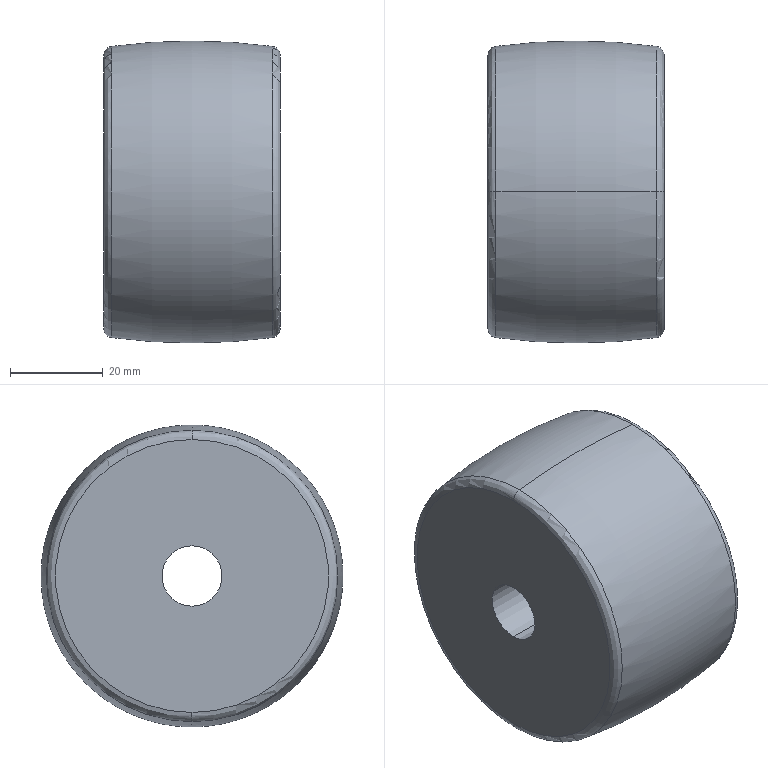Part | SolidWorks | features RefAxis 9, 3DProfileFeature 3, Revolution 1 | 1 solid | 10 faces | box 38 x 65 x 65 mm | volume 117321 mm3 | torus 6 | plane 2 | cylinder 2 | commonest cylinder face diameters 13 x2
STEP:
#1=CARTESIAN_POINT('',(-17.261,0.,31.371));
#2=VERTEX_POINT('',#1);
#3=CARTESIAN_POINT('',(-17.261,0.,-31.371));
#4=VERTEX_POINT('',#3);
#5=CARTESIAN_POINT('',(-17.261,0.,0.));
#6=DIRECTION('',(-1.,0.,0.));
#7=DIRECTION('',(0.,0.,1.));
#8=AXIS2_PLACEMENT_3D('',#5,#6,#7);
#9=CIRCLE('',#8,31.371);
#10=EDGE_CURVE('',#2,#4,#9,.T.);
#11=ORIENTED_EDGE('',*,*,#10,.T.);
#12=CARTESIAN_POINT('',(-19.,0.,-29.388));
#13=VERTEX_POINT('',#12);
#14=CARTESIAN_POINT('',(-17.,0.,-29.388));
#15=DIRECTION('',(0.,1.,0.));
#16=DIRECTION('',(0.,0.,1.));
#17=AXIS2_PLACEMENT_3D('',#14,#15,#16);
#18=CIRCLE('',#17,2.);
#19=EDGE_CURVE('',#4,#13,#18,.T.);
#20=ORIENTED_EDGE('',*,*,#19,.T.);
#21=CARTESIAN_POINT('',(-19.,0.,29.388));
#22=VERTEX_POINT('',#21);
#23=CARTESIAN_POINT('',(-19.,0.,0.));
#24=DIRECTION('',(-1.,0.,0.));
#25=DIRECTION('',(0.,0.,1.));
#26=AXIS2_PLACEMENT_3D('',#23,#24,#25);
#27=CIRCLE('',#26,29.388);
#28=EDGE_CURVE('',#22,#13,#27,.T.);
#29=ORIENTED_EDGE('',*,*,#28,.F.);
#30=CARTESIAN_POINT('',(-17.,0.,29.388));
#31=DIRECTION('',(0.,-1.,0.));
#32=DIRECTION('',(0.,0.,-1.));
#33=AXIS2_PLACEMENT_3D('',#30,#31,#32);
#34=CIRCLE('',#33,2.);
#35=EDGE_CURVE('',#2,#22,#34,.T.);
#36=ORIENTED_EDGE('',*,*,#35,.F.);
#37=EDGE_LOOP('',(#11,#20,#29,#36));
#38=FACE_OUTER_BOUND('',#37,.T.);
#39=CARTESIAN_POINT('',(-17.,0.,0.));
#40=DIRECTION('',(-1.,0.,0.));
#41=DIRECTION('',(0.,0.,1.));
#42=AXIS2_PLACEMENT_3D('',#39,#40,#41);
#43=TOROIDAL_SURFACE('',#42,29.388,2.);
#44=ADVANCED_FACE('',(#38),#43,.T.);
#45=CARTESIAN_POINT('',(17.261,0.,31.371));
#46=VERTEX_POINT('',#45);
#47=CARTESIAN_POINT('',(17.261,0.,-31.371));
#48=VERTEX_POINT('',#47);
#49=CARTESIAN_POINT('',(17.261,0.,0.));
#50=DIRECTION('',(-1.,0.,0.));
#51=DIRECTION('',(0.,0.,1.));
#52=AXIS2_PLACEMENT_3D('',#49,#50,#51);
#53=CIRCLE('',#52,31.371);
#54=EDGE_CURVE('',#46,#48,#53,.T.);
#55=ORIENTED_EDGE('',*,*,#54,.T.);
#56=CARTESIAN_POINT('',(0.,0.,100.));
#57=DIRECTION('',(0.,1.,0.));
#58=DIRECTION('',(0.,0.,1.));
#59=AXIS2_PLACEMENT_3D('',#56,#57,#58);
#60=CIRCLE('',#59,132.5);
#61=EDGE_CURVE('',#48,#4,#60,.T.);
#62=ORIENTED_EDGE('',*,*,#61,.T.);
#63=ORIENTED_EDGE('',*,*,#10,.F.);
#64=CARTESIAN_POINT('',(0.,0.,-100.));
#65=DIRECTION('',(0.,-1.,0.));
#66=DIRECTION('',(0.,0.,-1.));
#67=AXIS2_PLACEMENT_3D('',#64,#65,#66);
#68=CIRCLE('',#67,132.5);
#69=EDGE_CURVE('',#46,#2,#68,.T.);
#70=ORIENTED_EDGE('',*,*,#69,.F.);
#71=EDGE_LOOP('',(#55,#62,#63,#70));
#72=FACE_OUTER_BOUND('',#71,.T.);
#73=CARTESIAN_POINT('',(0.,0.,0.));
#74=DIRECTION('',(-1.,0.,0.));
#75=DIRECTION('',(0.,0.,1.));
#76=AXIS2_PLACEMENT_3D('',#73,#74,#75);
#77=TOROIDAL_SURFACE('',#76,-100.,132.5);
#78=ADVANCED_FACE('',(#72),#77,.T.);
#79=CARTESIAN_POINT('',(19.,0.,29.388));
#80=VERTEX_POINT('',#79);
#81=CARTESIAN_POINT('',(19.,0.,-29.388));
#82=VERTEX_POINT('',#81);
#83=CARTESIAN_POINT('',(19.,0.,0.));
#84=DIRECTION('',(-1.,0.,0.));
#85=DIRECTION('',(0.,0.,1.));
#86=AXIS2_PLACEMENT_3D('',#83,#84,#85);
#87=CIRCLE('',#86,29.388);
#88=EDGE_CURVE('',#80,#82,#87,.T.);
#89=ORIENTED_EDGE('',*,*,#88,.T.);
#90=CARTESIAN_POINT('',(17.,0.,-29.388));
#91=DIRECTION('',(0.,1.,0.));
#92=DIRECTION('',(0.,0.,1.));
#93=AXIS2_PLACEMENT_3D('',#90,#91,#92);
#94=CIRCLE('',#93,2.);
#95=EDGE_CURVE('',#82,#48,#94,.T.);
#96=ORIENTED_EDGE('',*,*,#95,.T.);
#97=ORIENTED_EDGE('',*,*,#54,.F.);
#98=CARTESIAN_POINT('',(17.,0.,29.388));
#99=DIRECTION('',(0.,-1.,0.));
#100=DIRECTION('',(0.,0.,-1.));
#101=AXIS2_PLACEMENT_3D('',#98,#99,#100);
#102=CIRCLE('',#101,2.);
#103=EDGE_CURVE('',#80,#46,#102,.T.);
#104=ORIENTED_EDGE('',*,*,#103,.F.);
#105=EDGE_LOOP('',(#89,#96,#97,#104));
#106=FACE_OUTER_BOUND('',#105,.T.);
#107=CARTESIAN_POINT('',(17.,0.,0.));
#108=DIRECTION('',(-1.,0.,0.));
#109=DIRECTION('',(0.,0.,1.));
#110=AXIS2_PLACEMENT_3D('',#107,#108,#109);
#111=TOROIDAL_SURFACE('',#110,29.388,2.);
#112=ADVANCED_FACE('',(#106),#111,.T.);
#113=CARTESIAN_POINT('',(19.,0.,-6.5));
#114=VERTEX_POINT('',#113);
#115=CARTESIAN_POINT('',(19.,0.,6.5));
#116=VERTEX_POINT('',#115);
#117=CARTESIAN_POINT('',(19.,0.,0.));
#118=DIRECTION('',(-1.,0.,0.));
#119=DIRECTION('',(0.,0.,1.));
#120=AXIS2_PLACEMENT_3D('',#117,#118,#119);
#121=CIRCLE('',#120,6.5);
#122=EDGE_CURVE('',#114,#116,#121,.T.);
#123=ORIENTED_EDGE('',*,*,#122,.F.);
#124=CARTESIAN_POINT('',(-19.,0.,-6.5));
#125=VERTEX_POINT('',#124);
#126=CARTESIAN_POINT('',(50.,0.,-6.5));
#127=DIRECTION('',(-1.,0.,0.));
#128=VECTOR('',#127,1000.);
#129=LINE('',#126,#128);
#130=EDGE_CURVE('',#114,#125,#129,.T.);
#131=ORIENTED_EDGE('',*,*,#130,.T.);
#132=CARTESIAN_POINT('',(-19.,0.,6.5));
#133=VERTEX_POINT('',#132);
#134=CARTESIAN_POINT('',(-19.,0.,0.));
#135=DIRECTION('',(-1.,0.,0.));
#136=DIRECTION('',(0.,0.,1.));
#137=AXIS2_PLACEMENT_3D('',#134,#135,#136);
#138=CIRCLE('',#137,6.5);
#139=EDGE_CURVE('',#125,#133,#138,.T.);
#140=ORIENTED_EDGE('',*,*,#139,.T.);
#141=CARTESIAN_POINT('',(50.,0.,6.5));
#142=DIRECTION('',(-1.,0.,0.));
#143=VECTOR('',#142,1000.);
#144=LINE('',#141,#143);
#145=EDGE_CURVE('',#116,#133,#144,.T.);
#146=ORIENTED_EDGE('',*,*,#145,.F.);
#147=EDGE_LOOP('',(#123,#131,#140,#146));
#148=FACE_OUTER_BOUND('',#147,.T.);
#149=CARTESIAN_POINT('',(50.,0.,0.));
#150=DIRECTION('',(-1.,0.,0.));
#151=DIRECTION('',(0.,0.,1.));
#152=AXIS2_PLACEMENT_3D('',#149,#150,#151);
#153=CYLINDRICAL_SURFACE('',#152,6.5);
#154=ADVANCED_FACE('',(#148),#153,.F.);
#155=CARTESIAN_POINT('',(-19.,0.,0.));
#156=DIRECTION('',(-1.,0.,0.));
#157=DIRECTION('',(0.,0.,1.));
#158=AXIS2_PLACEMENT_3D('',#155,#156,#157);
#159=CIRCLE('',#158,6.5);
#160=EDGE_CURVE('',#133,#125,#159,.T.);
#161=ORIENTED_EDGE('',*,*,#160,.F.);
#162=ORIENTED_EDGE('',*,*,#139,.F.);
#163=EDGE_LOOP('',(#161,#162));
#164=FACE_BOUND('',#163,.T.);
#165=ORIENTED_EDGE('',*,*,#28,.T.);
#166=CARTESIAN_POINT('',(-19.,0.,0.));
#167=DIRECTION('',(-1.,0.,0.));
#168=DIRECTION('',(0.,0.,1.));
#169=AXIS2_PLACEMENT_3D('',#166,#167,#168);
#170=CIRCLE('',#169,29.388);
#171=EDGE_CURVE('',#13,#22,#170,.T.);
#172=ORIENTED_EDGE('',*,*,#171,.T.);
#173=EDGE_LOOP('',(#165,#172));
#174=FACE_OUTER_BOUND('',#173,.T.);
#175=CARTESIAN_POINT('',(-19.,29.388,0.));
#176=DIRECTION('',(1.,0.,0.));
#177=DIRECTION('',(0.,0.,-1.));
#178=AXIS2_PLACEMENT_3D('',#175,#176,#177);
#179=PLANE('',#178);
#180=ADVANCED_FACE('',(#164,#174),#179,.F.);
#181=ORIENTED_EDGE('',*,*,#130,.F.);
#182=CARTESIAN_POINT('',(19.,0.,0.));
#183=DIRECTION('',(-1.,0.,0.));
#184=DIRECTION('',(0.,0.,1.));
#185=AXIS2_PLACEMENT_3D('',#182,#183,#184);
#186=CIRCLE('',#185,6.5);
#187=EDGE_CURVE('',#116,#114,#186,.T.);
#188=ORIENTED_EDGE('',*,*,#187,.F.);
#189=ORIENTED_EDGE('',*,*,#145,.T.);
#190=ORIENTED_EDGE('',*,*,#160,.T.);
#191=EDGE_LOOP('',(#181,#188,#189,#190));
#192=FACE_OUTER_BOUND('',#191,.T.);
#193=CARTESIAN_POINT('',(50.,0.,0.));
#194=DIRECTION('',(-1.,0.,0.));
#195=DIRECTION('',(0.,0.,1.));
#196=AXIS2_PLACEMENT_3D('',#193,#194,#195);
#197=CYLINDRICAL_SURFACE('',#196,6.5);
#198=ADVANCED_FACE('',(#192),#197,.F.);
#199=ORIENTED_EDGE('',*,*,#88,.F.);
#200=CARTESIAN_POINT('',(19.,0.,0.));
#201=DIRECTION('',(-1.,0.,0.));
#202=DIRECTION('',(0.,0.,1.));
#203=AXIS2_PLACEMENT_3D('',#200,#201,#202);
#204=CIRCLE('',#203,29.388);
#205=EDGE_CURVE('',#82,#80,#204,.T.);
#206=ORIENTED_EDGE('',*,*,#205,.F.);
#207=EDGE_LOOP('',(#199,#206));
#208=FACE_OUTER_BOUND('',#207,.T.);
#209=ORIENTED_EDGE('',*,*,#187,.T.);
#210=ORIENTED_EDGE('',*,*,#122,.T.);
#211=EDGE_LOOP('',(#209,#210));
#212=FACE_BOUND('',#211,.T.);
#213=CARTESIAN_POINT('',(19.,6.5,0.));
#214=DIRECTION('',(-1.,0.,0.));
#215=DIRECTION('',(0.,0.,1.));
#216=AXIS2_PLACEMENT_3D('',#213,#214,#215);
#217=PLANE('',#216);
#218=ADVANCED_FACE('',(#208,#212),#217,.F.);
#219=ORIENTED_EDGE('',*,*,#95,.F.);
#220=ORIENTED_EDGE('',*,*,#205,.T.);
#221=ORIENTED_EDGE('',*,*,#103,.T.);
#222=CARTESIAN_POINT('',(17.261,0.,0.));
#223=DIRECTION('',(-1.,0.,0.));
#224=DIRECTION('',(0.,0.,1.));
#225=AXIS2_PLACEMENT_3D('',#222,#223,#224);
#226=CIRCLE('',#225,31.371);
#227=EDGE_CURVE('',#48,#46,#226,.T.);
#228=ORIENTED_EDGE('',*,*,#227,.F.);
#229=EDGE_LOOP('',(#219,#220,#221,#228));
#230=FACE_OUTER_BOUND('',#229,.T.);
#231=CARTESIAN_POINT('',(17.,0.,0.));
#232=DIRECTION('',(-1.,0.,0.));
#233=DIRECTION('',(0.,0.,1.));
#234=AXIS2_PLACEMENT_3D('',#231,#232,#233);
#235=TOROIDAL_SURFACE('',#234,29.388,2.);
#236=ADVANCED_FACE('',(#230),#235,.T.);
#237=ORIENTED_EDGE('',*,*,#61,.F.);
#238=ORIENTED_EDGE('',*,*,#227,.T.);
#239=ORIENTED_EDGE('',*,*,#69,.T.);
#240=CARTESIAN_POINT('',(-17.261,0.,0.));
#241=DIRECTION('',(-1.,0.,0.));
#242=DIRECTION('',(0.,0.,1.));
#243=AXIS2_PLACEMENT_3D('',#240,#241,#242);
#244=CIRCLE('',#243,31.371);
#245=EDGE_CURVE('',#4,#2,#244,.T.);
#246=ORIENTED_EDGE('',*,*,#245,.F.);
#247=EDGE_LOOP('',(#237,#238,#239,#246));
#248=FACE_OUTER_BOUND('',#247,.T.);
#249=CARTESIAN_POINT('',(0.,0.,0.));
#250=DIRECTION('',(-1.,0.,0.));
#251=DIRECTION('',(0.,0.,1.));
#252=AXIS2_PLACEMENT_3D('',#249,#250,#251);
#253=TOROIDAL_SURFACE('',#252,-100.,132.5);
#254=ADVANCED_FACE('',(#248),#253,.T.);
#255=ORIENTED_EDGE('',*,*,#19,.F.);
#256=ORIENTED_EDGE('',*,*,#245,.T.);
#257=ORIENTED_EDGE('',*,*,#35,.T.);
#258=ORIENTED_EDGE('',*,*,#171,.F.);
#259=EDGE_LOOP('',(#255,#256,#257,#258));
#260=FACE_OUTER_BOUND('',#259,.T.);
#261=CARTESIAN_POINT('',(-17.,0.,0.));
#262=DIRECTION('',(-1.,0.,0.));
#263=DIRECTION('',(0.,0.,1.));
#264=AXIS2_PLACEMENT_3D('',#261,#262,#263);
#265=TOROIDAL_SURFACE('',#264,29.388,2.);
#266=ADVANCED_FACE('',(#260),#265,.T.);
#267=CLOSED_SHELL('',(#44,#78,#112,#154,#180,#198,#218,#236,#254,#266));
#268=MANIFOLD_SOLID_BREP('',#267);
#269=CARTESIAN_POINT('',(0.,0.,0.));
#270=DIRECTION('',(0.,0.,1.));
#271=DIRECTION('',(1.,0.,0.));
#272=AXIS2_PLACEMENT_3D('',#269,#270,#271);
#273=(LENGTH_UNIT()NAMED_UNIT(*)SI_UNIT(.MILLI.,.METRE.));
#274=UNCERTAINTY_MEASURE_WITH_UNIT(LENGTH_MEASURE(0.00001),#273,'','');
#275=(NAMED_UNIT(*)PLANE_ANGLE_UNIT()SI_UNIT($,.RADIAN.));
#276=(NAMED_UNIT(*)SI_UNIT($,.STERADIAN.)SOLID_ANGLE_UNIT());
#277=(GEOMETRIC_REPRESENTATION_CONTEXT(3)GLOBAL_UNCERTAINTY_ASSIGNED_CONTEXT((#274))GLOBAL_UNIT_ASSIGNED_CONTEXT((#273,#275,#276))REPRESENTATION_CONTEXT('',''));
#278=ADVANCED_BREP_SHAPE_REPRESENTATION('',(#268,#272),#277);